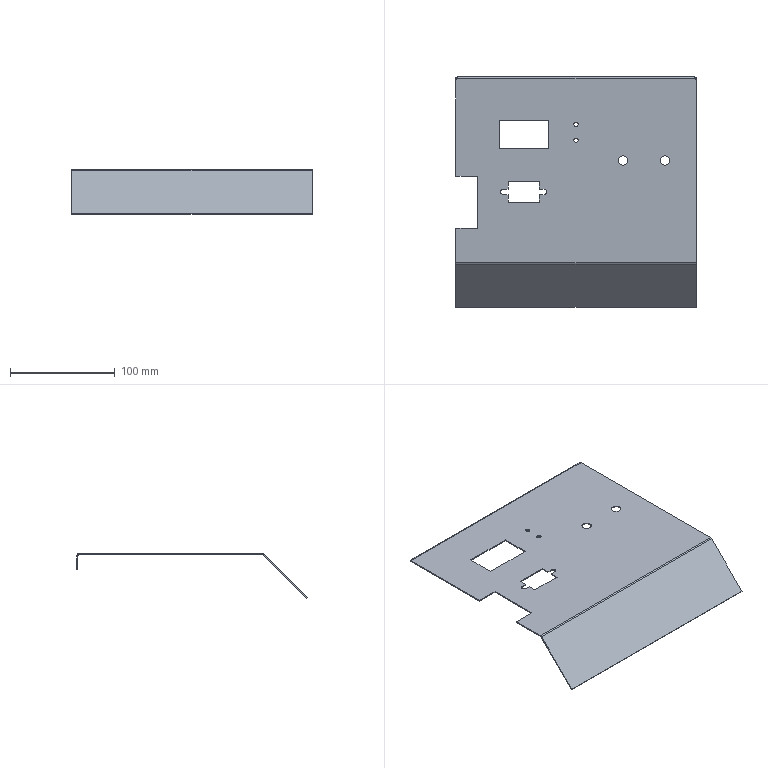Part | SolidWorks | features BaseBody 1 | 1 solid | 59 faces | box 230 x 220.134 x 42.426 mm | volume 54204 mm3 | plane 42 | cylinder 15 | spline 2 | commonest cylinder face diameters 4 x6 9 x4 5 x3 2 x2